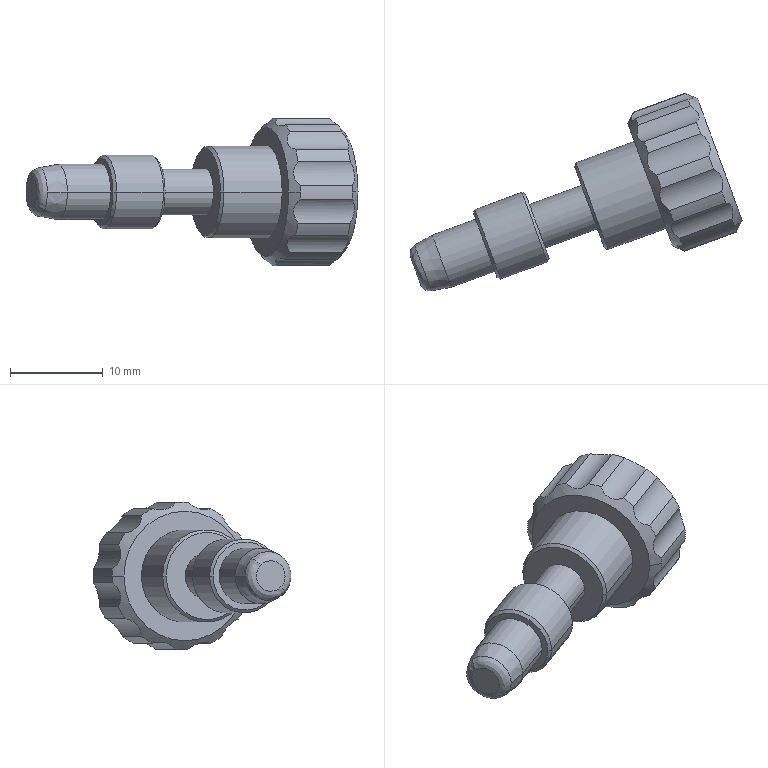Part | SolidWorks | features BaseBody 1 | 1 solid | 55 faces | box 35.902 x 21.412 x 16 mm | volume 2667 mm3 | cylinder 35 | cone 12 | plane 6 | spline 2 | commonest cylinder face diameters 5 x16 16 x13 6 x2 8 x2 10 x2